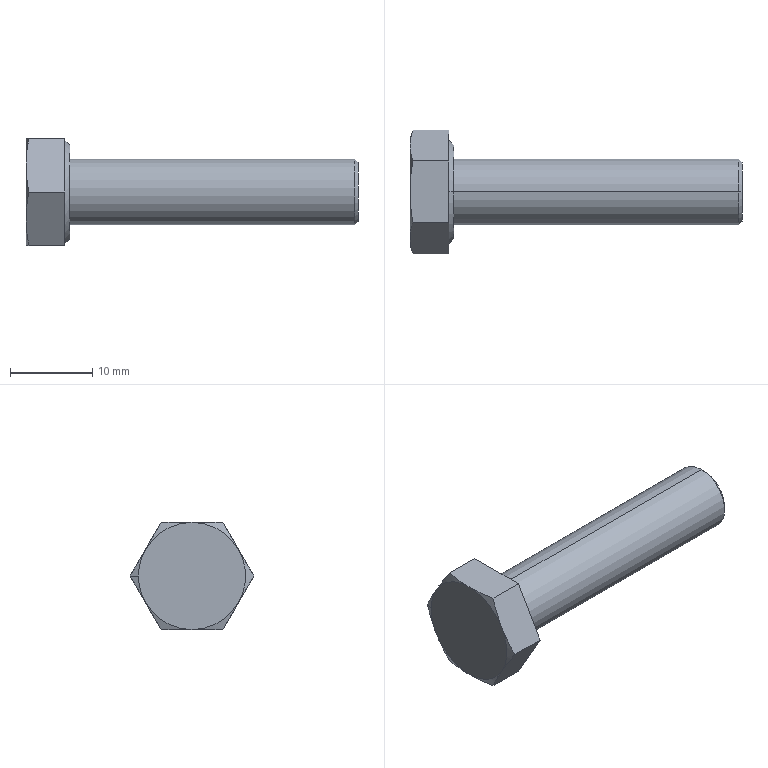Part | STEP file | hex head bolts-full thread grade c gb_GB_FASTENER_BOLT_HHBFTC M8X35-S | 1 solid | 23 faces | box 40.3 x 15.011 x 13 mm | volume 2512 mm3 | cone 11 | plane 10 | cylinder 2 | commonest cylinder face diameters 8 x2
STEP:
#1=CARTESIAN_POINT('',(39.9,0.,4.));
#2=VERTEX_POINT('',#1);
#3=CARTESIAN_POINT('',(39.9,0.,-4.));
#4=VERTEX_POINT('',#3);
#5=CARTESIAN_POINT('',(39.9,0.,0.));
#6=DIRECTION('',(-1.,0.,0.));
#7=DIRECTION('',(0.,0.,1.));
#8=AXIS2_PLACEMENT_3D('',#5,#6,#7);
#9=CIRCLE('',#8,4.);
#10=EDGE_CURVE('',#2,#4,#9,.T.);
#11=ORIENTED_EDGE('',*,*,#10,.T.);
#12=CARTESIAN_POINT('',(5.3,0.,-4.));
#13=VERTEX_POINT('',#12);
#14=CARTESIAN_POINT('',(40.3,0.,-4.));
#15=DIRECTION('',(-1.,0.,0.));
#16=VECTOR('',#15,1000.);
#17=LINE('',#14,#16);
#18=EDGE_CURVE('',#4,#13,#17,.T.);
#19=ORIENTED_EDGE('',*,*,#18,.T.);
#20=CARTESIAN_POINT('',(5.3,0.,4.));
#21=VERTEX_POINT('',#20);
#22=CARTESIAN_POINT('',(5.3,0.,0.));
#23=DIRECTION('',(1.,0.,0.));
#24=DIRECTION('',(0.,0.,1.));
#25=AXIS2_PLACEMENT_3D('',#22,#23,#24);
#26=CIRCLE('',#25,4.);
#27=EDGE_CURVE('',#13,#21,#26,.T.);
#28=ORIENTED_EDGE('',*,*,#27,.T.);
#29=CARTESIAN_POINT('',(40.3,0.,4.));
#30=DIRECTION('',(-1.,0.,0.));
#31=VECTOR('',#30,1000.);
#32=LINE('',#29,#31);
#33=EDGE_CURVE('',#2,#21,#32,.T.);
#34=ORIENTED_EDGE('',*,*,#33,.F.);
#35=EDGE_LOOP('',(#11,#19,#28,#34));
#36=FACE_OUTER_BOUND('',#35,.T.);
#37=CARTESIAN_POINT('',(40.3,0.,0.));
#38=DIRECTION('',(-1.,0.,0.));
#39=DIRECTION('',(0.,0.,1.));
#40=AXIS2_PLACEMENT_3D('',#37,#38,#39);
#41=CYLINDRICAL_SURFACE('',#40,4.);
#42=ADVANCED_FACE('',(#36),#41,.T.);
#43=CARTESIAN_POINT('',(40.3,0.,3.6));
#44=VERTEX_POINT('',#43);
#45=CARTESIAN_POINT('',(40.3,0.,-3.6));
#46=VERTEX_POINT('',#45);
#47=CARTESIAN_POINT('',(40.3,0.,0.));
#48=DIRECTION('',(-1.,0.,0.));
#49=DIRECTION('',(0.,0.,1.));
#50=AXIS2_PLACEMENT_3D('',#47,#48,#49);
#51=CIRCLE('',#50,3.6);
#52=EDGE_CURVE('',#44,#46,#51,.T.);
#53=ORIENTED_EDGE('',*,*,#52,.T.);
#54=CARTESIAN_POINT('',(39.9,0.,-4.));
#55=DIRECTION('',(-0.7071,0.,-0.7071));
#56=VECTOR('',#55,1000.);
#57=LINE('',#54,#56);
#58=EDGE_CURVE('',#46,#4,#57,.T.);
#59=ORIENTED_EDGE('',*,*,#58,.T.);
#60=ORIENTED_EDGE('',*,*,#10,.F.);
#61=CARTESIAN_POINT('',(39.9,0.,4.));
#62=DIRECTION('',(-0.7071,0.,0.7071));
#63=VECTOR('',#62,1000.);
#64=LINE('',#61,#63);
#65=EDGE_CURVE('',#44,#2,#64,.T.);
#66=ORIENTED_EDGE('',*,*,#65,.F.);
#67=EDGE_LOOP('',(#53,#59,#60,#66));
#68=FACE_OUTER_BOUND('',#67,.T.);
#69=CARTESIAN_POINT('',(39.9,0.,0.));
#70=DIRECTION('',(-1.,0.,0.));
#71=DIRECTION('',(0.,0.,1.));
#72=AXIS2_PLACEMENT_3D('',#69,#70,#71);
#73=CONICAL_SURFACE('',#72,4.,0.7854);
#74=ADVANCED_FACE('',(#68),#73,.T.);
#75=CARTESIAN_POINT('',(5.3,0.,-5.735));
#76=VERTEX_POINT('',#75);
#77=CARTESIAN_POINT('',(5.3,0.,5.735));
#78=VERTEX_POINT('',#77);
#79=CARTESIAN_POINT('',(5.3,0.,0.));
#80=DIRECTION('',(1.,0.,0.));
#81=DIRECTION('',(0.,0.,1.));
#82=AXIS2_PLACEMENT_3D('',#79,#80,#81);
#83=CIRCLE('',#82,5.735);
#84=EDGE_CURVE('',#76,#78,#83,.T.);
#85=ORIENTED_EDGE('',*,*,#84,.F.);
#86=CARTESIAN_POINT('',(4.7,0.,-6.335));
#87=VERTEX_POINT('',#86);
#88=CARTESIAN_POINT('',(4.7,0.,-6.335));
#89=DIRECTION('',(-0.7071,0.,-0.7071));
#90=VECTOR('',#89,1000.);
#91=LINE('',#88,#90);
#92=EDGE_CURVE('',#76,#87,#91,.T.);
#93=ORIENTED_EDGE('',*,*,#92,.T.);
#94=CARTESIAN_POINT('',(4.7,0.,6.335));
#95=VERTEX_POINT('',#94);
#96=CARTESIAN_POINT('',(4.7,0.,0.));
#97=DIRECTION('',(1.,0.,0.));
#98=DIRECTION('',(0.,0.,1.));
#99=AXIS2_PLACEMENT_3D('',#96,#97,#98);
#100=CIRCLE('',#99,6.335);
#101=EDGE_CURVE('',#87,#95,#100,.T.);
#102=ORIENTED_EDGE('',*,*,#101,.T.);
#103=CARTESIAN_POINT('',(4.7,0.,6.335));
#104=DIRECTION('',(-0.7071,0.,0.7071));
#105=VECTOR('',#104,1000.);
#106=LINE('',#103,#105);
#107=EDGE_CURVE('',#78,#95,#106,.T.);
#108=ORIENTED_EDGE('',*,*,#107,.F.);
#109=EDGE_LOOP('',(#85,#93,#102,#108));
#110=FACE_OUTER_BOUND('',#109,.T.);
#111=CARTESIAN_POINT('',(4.7,0.,0.));
#112=DIRECTION('',(-1.,0.,0.));
#113=DIRECTION('',(0.,0.,1.));
#114=AXIS2_PLACEMENT_3D('',#111,#112,#113);
#115=CONICAL_SURFACE('',#114,6.335,0.7854);
#116=ADVANCED_FACE('',(#110),#115,.T.);
#117=CARTESIAN_POINT('',(0.,5.629,-3.25));
#118=VERTEX_POINT('',#117);
#119=CARTESIAN_POINT('',(0.,6.5,0.));
#120=VERTEX_POINT('',#119);
#121=CARTESIAN_POINT('',(0.,0.,0.));
#122=DIRECTION('',(1.,0.,0.));
#123=DIRECTION('',(0.,1.,0.));
#124=AXIS2_PLACEMENT_3D('',#121,#122,#123);
#125=CIRCLE('',#124,6.5);
#126=EDGE_CURVE('',#118,#120,#125,.T.);
#127=ORIENTED_EDGE('',*,*,#126,.T.);
#128=CARTESIAN_POINT('',(0.366,7.506,0.));
#129=VERTEX_POINT('',#128);
#130=CARTESIAN_POINT('',(0.3682,7.512,0.));
#131=DIRECTION('',(0.342,0.9397,0.));
#132=VECTOR('',#131,1000.);
#133=LINE('',#130,#132);
#134=EDGE_CURVE('',#120,#129,#133,.T.);
#135=ORIENTED_EDGE('',*,*,#134,.T.);
#136=CARTESIAN_POINT('',(0.366,7.506,0.));
#137=CARTESIAN_POINT('',(0.1402,6.885,-1.075));
#138=CARTESIAN_POINT('',(0.,6.261,-2.156));
#139=CARTESIAN_POINT('',(0.,5.629,-3.25));
#140=B_SPLINE_CURVE_WITH_KNOTS('',3,(#136,#137,#138,#139),.UNSPECIFIED.,.F.,.F.,(4,4),(0.,0.003771),.UNSPECIFIED.);
#141=EDGE_CURVE('',#129,#118,#140,.T.);
#142=ORIENTED_EDGE('',*,*,#141,.T.);
#143=EDGE_LOOP('',(#127,#135,#142));
#144=FACE_OUTER_BOUND('',#143,.T.);
#145=CARTESIAN_POINT('',(0.3682,0.,0.));
#146=DIRECTION('',(1.,0.,0.));
#147=DIRECTION('',(0.,1.,0.));
#148=AXIS2_PLACEMENT_3D('',#145,#146,#147);
#149=CONICAL_SURFACE('',#148,7.512,1.222);
#150=ADVANCED_FACE('',(#144),#149,.T.);
#151=ORIENTED_EDGE('',*,*,#18,.F.);
#152=CARTESIAN_POINT('',(39.9,0.,0.));
#153=DIRECTION('',(-1.,0.,0.));
#154=DIRECTION('',(0.,0.,1.));
#155=AXIS2_PLACEMENT_3D('',#152,#153,#154);
#156=CIRCLE('',#155,4.);
#157=EDGE_CURVE('',#4,#2,#156,.T.);
#158=ORIENTED_EDGE('',*,*,#157,.T.);
#159=ORIENTED_EDGE('',*,*,#33,.T.);
#160=CARTESIAN_POINT('',(5.3,0.,0.));
#161=DIRECTION('',(1.,0.,0.));
#162=DIRECTION('',(0.,0.,1.));
#163=AXIS2_PLACEMENT_3D('',#160,#161,#162);
#164=CIRCLE('',#163,4.);
#165=EDGE_CURVE('',#21,#13,#164,.T.);
#166=ORIENTED_EDGE('',*,*,#165,.T.);
#167=EDGE_LOOP('',(#151,#158,#159,#166));
#168=FACE_OUTER_BOUND('',#167,.T.);
#169=CARTESIAN_POINT('',(40.3,0.,0.));
#170=DIRECTION('',(-1.,0.,0.));
#171=DIRECTION('',(0.,0.,1.));
#172=AXIS2_PLACEMENT_3D('',#169,#170,#171);
#173=CYLINDRICAL_SURFACE('',#172,4.);
#174=ADVANCED_FACE('',(#168),#173,.T.);
#175=ORIENTED_EDGE('',*,*,#165,.F.);
#176=ORIENTED_EDGE('',*,*,#27,.F.);
#177=EDGE_LOOP('',(#175,#176));
#178=FACE_BOUND('',#177,.T.);
#179=CARTESIAN_POINT('',(5.3,0.,0.));
#180=DIRECTION('',(1.,0.,0.));
#181=DIRECTION('',(0.,0.,1.));
#182=AXIS2_PLACEMENT_3D('',#179,#180,#181);
#183=CIRCLE('',#182,5.735);
#184=EDGE_CURVE('',#78,#76,#183,.T.);
#185=ORIENTED_EDGE('',*,*,#184,.T.);
#186=ORIENTED_EDGE('',*,*,#84,.T.);
#187=EDGE_LOOP('',(#185,#186));
#188=FACE_OUTER_BOUND('',#187,.T.);
#189=CARTESIAN_POINT('',(5.3,-7.506,0.));
#190=DIRECTION('',(1.,0.,0.));
#191=DIRECTION('',(0.,0.,-1.));
#192=AXIS2_PLACEMENT_3D('',#189,#190,#191);
#193=PLANE('',#192);
#194=ADVANCED_FACE('',(#178,#188),#193,.T.);
#195=ORIENTED_EDGE('',*,*,#58,.F.);
#196=CARTESIAN_POINT('',(40.3,0.,0.));
#197=DIRECTION('',(-1.,0.,0.));
#198=DIRECTION('',(0.,0.,1.));
#199=AXIS2_PLACEMENT_3D('',#196,#197,#198);
#200=CIRCLE('',#199,3.6);
#201=EDGE_CURVE('',#46,#44,#200,.T.);
#202=ORIENTED_EDGE('',*,*,#201,.T.);
#203=ORIENTED_EDGE('',*,*,#65,.T.);
#204=ORIENTED_EDGE('',*,*,#157,.F.);
#205=EDGE_LOOP('',(#195,#202,#203,#204));
#206=FACE_OUTER_BOUND('',#205,.T.);
#207=CARTESIAN_POINT('',(39.9,0.,0.));
#208=DIRECTION('',(-1.,0.,0.));
#209=DIRECTION('',(0.,0.,1.));
#210=AXIS2_PLACEMENT_3D('',#207,#208,#209);
#211=CONICAL_SURFACE('',#210,4.,0.7854);
#212=ADVANCED_FACE('',(#206),#211,.T.);
#213=ORIENTED_EDGE('',*,*,#92,.F.);
#214=ORIENTED_EDGE('',*,*,#184,.F.);
#215=ORIENTED_EDGE('',*,*,#107,.T.);
#216=CARTESIAN_POINT('',(4.7,0.,0.));
#217=DIRECTION('',(1.,0.,0.));
#218=DIRECTION('',(0.,0.,1.));
#219=AXIS2_PLACEMENT_3D('',#216,#217,#218);
#220=CIRCLE('',#219,6.335);
#221=EDGE_CURVE('',#95,#87,#220,.T.);
#222=ORIENTED_EDGE('',*,*,#221,.T.);
#223=EDGE_LOOP('',(#213,#214,#215,#222));
#224=FACE_OUTER_BOUND('',#223,.T.);
#225=CARTESIAN_POINT('',(4.7,0.,0.));
#226=DIRECTION('',(-1.,0.,0.));
#227=DIRECTION('',(0.,0.,1.));
#228=AXIS2_PLACEMENT_3D('',#225,#226,#227);
#229=CONICAL_SURFACE('',#228,6.335,0.7854);
#230=ADVANCED_FACE('',(#224),#229,.T.);
#231=ORIENTED_EDGE('',*,*,#52,.F.);
#232=ORIENTED_EDGE('',*,*,#201,.F.);
#233=EDGE_LOOP('',(#231,#232));
#234=FACE_OUTER_BOUND('',#233,.T.);
#235=CARTESIAN_POINT('',(40.3,0.,0.));
#236=DIRECTION('',(1.,0.,0.));
#237=DIRECTION('',(0.,0.,-1.));
#238=AXIS2_PLACEMENT_3D('',#235,#236,#237);
#239=PLANE('',#238);
#240=ADVANCED_FACE('',(#234),#239,.T.);
#241=CARTESIAN_POINT('',(4.7,7.506,0.));
#242=VERTEX_POINT('',#241);
#243=CARTESIAN_POINT('',(4.7,3.753,6.5));
#244=VERTEX_POINT('',#243);
#245=CARTESIAN_POINT('',(4.7,7.506,0.));
#246=DIRECTION('',(0.,-0.5,0.866));
#247=VECTOR('',#246,1000.);
#248=LINE('',#245,#247);
#249=EDGE_CURVE('',#242,#244,#248,.T.);
#250=ORIENTED_EDGE('',*,*,#249,.T.);
#251=CARTESIAN_POINT('',(4.7,-3.753,6.5));
#252=VERTEX_POINT('',#251);
#253=CARTESIAN_POINT('',(4.7,6.335,6.5));
#254=DIRECTION('',(0.,-1.,0.));
#255=VECTOR('',#254,1000.);
#256=LINE('',#253,#255);
#257=EDGE_CURVE('',#244,#252,#256,.T.);
#258=ORIENTED_EDGE('',*,*,#257,.T.);
#259=CARTESIAN_POINT('',(4.7,-7.506,0.));
#260=VERTEX_POINT('',#259);
#261=CARTESIAN_POINT('',(4.7,-3.753,6.5));
#262=DIRECTION('',(0.,-0.5,-0.866));
#263=VECTOR('',#262,1000.);
#264=LINE('',#261,#263);
#265=EDGE_CURVE('',#252,#260,#264,.T.);
#266=ORIENTED_EDGE('',*,*,#265,.T.);
#267=CARTESIAN_POINT('',(4.7,-3.753,-6.5));
#268=VERTEX_POINT('',#267);
#269=CARTESIAN_POINT('',(4.7,-7.506,0.));
#270=DIRECTION('',(0.,0.5,-0.866));
#271=VECTOR('',#270,1000.);
#272=LINE('',#269,#271);
#273=EDGE_CURVE('',#260,#268,#272,.T.);
#274=ORIENTED_EDGE('',*,*,#273,.T.);
#275=CARTESIAN_POINT('',(4.7,3.753,-6.5));
#276=VERTEX_POINT('',#275);
#277=CARTESIAN_POINT('',(4.7,6.335,-6.5));
#278=DIRECTION('',(0.,1.,0.));
#279=VECTOR('',#278,1000.);
#280=LINE('',#277,#279);
#281=EDGE_CURVE('',#268,#276,#280,.T.);
#282=ORIENTED_EDGE('',*,*,#281,.T.);
#283=CARTESIAN_POINT('',(4.7,3.753,-6.5));
#284=DIRECTION('',(0.,0.5,0.866));
#285=VECTOR('',#284,1000.);
#286=LINE('',#283,#285);
#287=EDGE_CURVE('',#276,#242,#286,.T.);
#288=ORIENTED_EDGE('',*,*,#287,.T.);
#289=EDGE_LOOP('',(#250,#258,#266,#274,#282,#288));
#290=FACE_OUTER_BOUND('',#289,.T.);
#291=ORIENTED_EDGE('',*,*,#221,.F.);
#292=ORIENTED_EDGE('',*,*,#101,.F.);
#293=EDGE_LOOP('',(#291,#292));
#294=FACE_BOUND('',#293,.T.);
#295=CARTESIAN_POINT('',(4.7,6.335,0.));
#296=DIRECTION('',(1.,0.,0.));
#297=DIRECTION('',(0.,0.,-1.));
#298=AXIS2_PLACEMENT_3D('',#295,#296,#297);
#299=PLANE('',#298);
#300=ADVANCED_FACE('',(#290,#294),#299,.T.);
#301=CARTESIAN_POINT('',(0.366,-3.753,6.5));
#302=VERTEX_POINT('',#301);
#303=CARTESIAN_POINT('',(5.3,-3.753,6.5));
#304=DIRECTION('',(-1.,0.,0.));
#305=VECTOR('',#304,1000.);
#306=LINE('',#303,#305);
#307=EDGE_CURVE('',#252,#302,#306,.T.);
#308=ORIENTED_EDGE('',*,*,#307,.F.);
#309=ORIENTED_EDGE('',*,*,#257,.F.);
#310=CARTESIAN_POINT('',(0.366,3.753,6.5));
#311=VERTEX_POINT('',#310);
#312=CARTESIAN_POINT('',(5.3,3.753,6.5));
#313=DIRECTION('',(1.,0.,0.));
#314=VECTOR('',#313,1000.);
#315=LINE('',#312,#314);
#316=EDGE_CURVE('',#311,#244,#315,.T.);
#317=ORIENTED_EDGE('',*,*,#316,.F.);
#318=CARTESIAN_POINT('',(0.,0.,6.5));
#319=VERTEX_POINT('',#318);
#320=CARTESIAN_POINT('',(0.,0.,6.5));
#321=CARTESIAN_POINT('',(0.,1.263,6.5));
#322=CARTESIAN_POINT('',(0.1402,2.512,6.5));
#323=CARTESIAN_POINT('',(0.366,3.753,6.5));
#324=B_SPLINE_CURVE_WITH_KNOTS('',3,(#320,#321,#322,#323),.UNSPECIFIED.,.F.,.F.,(4,4),(0.,0.003771),.UNSPECIFIED.);
#325=EDGE_CURVE('',#319,#311,#324,.T.);
#326=ORIENTED_EDGE('',*,*,#325,.F.);
#327=CARTESIAN_POINT('',(0.366,-3.753,6.5));
#328=CARTESIAN_POINT('',(0.1402,-2.512,6.5));
#329=CARTESIAN_POINT('',(0.,-1.263,6.5));
#330=CARTESIAN_POINT('',(0.,0.,6.5));
#331=B_SPLINE_CURVE_WITH_KNOTS('',3,(#327,#328,#329,#330),.UNSPECIFIED.,.F.,.F.,(4,4),(0.,0.003771),.UNSPECIFIED.);
#332=EDGE_CURVE('',#302,#319,#331,.T.);
#333=ORIENTED_EDGE('',*,*,#332,.F.);
#334=EDGE_LOOP('',(#308,#309,#317,#326,#333));
#335=FACE_OUTER_BOUND('',#334,.T.);
#336=CARTESIAN_POINT('',(5.3,3.753,6.5));
#337=DIRECTION('',(0.,0.,-1.));
#338=DIRECTION('',(-1.,0.,0.));
#339=AXIS2_PLACEMENT_3D('',#336,#337,#338);
#340=PLANE('',#339);
#341=ADVANCED_FACE('',(#335),#340,.F.);
#342=ORIENTED_EDGE('',*,*,#316,.T.);
#343=ORIENTED_EDGE('',*,*,#249,.F.);
#344=CARTESIAN_POINT('',(5.3,7.506,0.));
#345=DIRECTION('',(1.,0.,0.));
#346=VECTOR('',#345,1000.);
#347=LINE('',#344,#346);
#348=EDGE_CURVE('',#129,#242,#347,.T.);
#349=ORIENTED_EDGE('',*,*,#348,.F.);
#350=CARTESIAN_POINT('',(0.,5.629,3.25));
#351=VERTEX_POINT('',#350);
#352=CARTESIAN_POINT('',(0.,5.629,3.25));
#353=CARTESIAN_POINT('',(0.,6.261,2.156));
#354=CARTESIAN_POINT('',(0.1402,6.885,1.075));
#355=CARTESIAN_POINT('',(0.366,7.506,0.));
#356=B_SPLINE_CURVE_WITH_KNOTS('',3,(#352,#353,#354,#355),.UNSPECIFIED.,.F.,.F.,(4,4),(0.,0.003771),.UNSPECIFIED.);
#357=EDGE_CURVE('',#351,#129,#356,.T.);
#358=ORIENTED_EDGE('',*,*,#357,.F.);
#359=CARTESIAN_POINT('',(0.366,3.753,6.5));
#360=CARTESIAN_POINT('',(0.1402,4.373,5.425));
#361=CARTESIAN_POINT('',(0.,4.998,4.344));
#362=CARTESIAN_POINT('',(0.,5.629,3.25));
#363=B_SPLINE_CURVE_WITH_KNOTS('',3,(#359,#360,#361,#362),.UNSPECIFIED.,.F.,.F.,(4,4),(0.,0.003771),.UNSPECIFIED.);
#364=EDGE_CURVE('',#311,#351,#363,.T.);
#365=ORIENTED_EDGE('',*,*,#364,.F.);
#366=EDGE_LOOP('',(#342,#343,#349,#358,#365));
#367=FACE_OUTER_BOUND('',#366,.T.);
#368=CARTESIAN_POINT('',(5.3,7.506,0.));
#369=DIRECTION('',(0.,-0.866,-0.5));
#370=DIRECTION('',(0.,0.5,-0.866));
#371=AXIS2_PLACEMENT_3D('',#368,#369,#370);
#372=PLANE('',#371);
#373=ADVANCED_FACE('',(#367),#372,.F.);
#374=ORIENTED_EDGE('',*,*,#348,.T.);
#375=ORIENTED_EDGE('',*,*,#287,.F.);
#376=CARTESIAN_POINT('',(0.366,3.753,-6.5));
#377=VERTEX_POINT('',#376);
#378=CARTESIAN_POINT('',(5.3,3.753,-6.5));
#379=DIRECTION('',(1.,0.,0.));
#380=VECTOR('',#379,1000.);
#381=LINE('',#378,#380);
#382=EDGE_CURVE('',#377,#276,#381,.T.);
#383=ORIENTED_EDGE('',*,*,#382,.F.);
#384=CARTESIAN_POINT('',(0.,5.629,-3.25));
#385=CARTESIAN_POINT('',(0.,4.998,-4.344));
#386=CARTESIAN_POINT('',(0.1402,4.373,-5.425));
#387=CARTESIAN_POINT('',(0.366,3.753,-6.5));
#388=B_SPLINE_CURVE_WITH_KNOTS('',3,(#384,#385,#386,#387),.UNSPECIFIED.,.F.,.F.,(4,4),(0.,0.003771),.UNSPECIFIED.);
#389=EDGE_CURVE('',#118,#377,#388,.T.);
#390=ORIENTED_EDGE('',*,*,#389,.F.);
#391=ORIENTED_EDGE('',*,*,#141,.F.);
#392=EDGE_LOOP('',(#374,#375,#383,#390,#391));
#393=FACE_OUTER_BOUND('',#392,.T.);
#394=CARTESIAN_POINT('',(5.3,3.753,-6.5));
#395=DIRECTION('',(0.,-0.866,0.5));
#396=DIRECTION('',(0.,-0.5,-0.866));
#397=AXIS2_PLACEMENT_3D('',#394,#395,#396);
#398=PLANE('',#397);
#399=ADVANCED_FACE('',(#393),#398,.F.);
#400=ORIENTED_EDGE('',*,*,#382,.T.);
#401=ORIENTED_EDGE('',*,*,#281,.F.);
#402=CARTESIAN_POINT('',(0.366,-3.753,-6.5));
#403=VERTEX_POINT('',#402);
#404=CARTESIAN_POINT('',(5.3,-3.753,-6.5));
#405=DIRECTION('',(1.,0.,0.));
#406=VECTOR('',#405,1000.);
#407=LINE('',#404,#406);
#408=EDGE_CURVE('',#403,#268,#407,.T.);
#409=ORIENTED_EDGE('',*,*,#408,.F.);
#410=CARTESIAN_POINT('',(0.,0.,-6.5));
#411=VERTEX_POINT('',#410);
#412=CARTESIAN_POINT('',(0.,0.,-6.5));
#413=CARTESIAN_POINT('',(0.,-1.263,-6.5));
#414=CARTESIAN_POINT('',(0.1402,-2.512,-6.5));
#415=CARTESIAN_POINT('',(0.366,-3.753,-6.5));
#416=B_SPLINE_CURVE_WITH_KNOTS('',3,(#412,#413,#414,#415),.UNSPECIFIED.,.F.,.F.,(4,4),(0.,0.003771),.UNSPECIFIED.);
#417=EDGE_CURVE('',#411,#403,#416,.T.);
#418=ORIENTED_EDGE('',*,*,#417,.F.);
#419=CARTESIAN_POINT('',(0.366,3.753,-6.5));
#420=CARTESIAN_POINT('',(0.1402,2.512,-6.5));
#421=CARTESIAN_POINT('',(0.,1.263,-6.5));
#422=CARTESIAN_POINT('',(0.,0.,-6.5));
#423=B_SPLINE_CURVE_WITH_KNOTS('',3,(#419,#420,#421,#422),.UNSPECIFIED.,.F.,.F.,(4,4),(0.,0.003771),.UNSPECIFIED.);
#424=EDGE_CURVE('',#377,#411,#423,.T.);
#425=ORIENTED_EDGE('',*,*,#424,.F.);
#426=EDGE_LOOP('',(#400,#401,#409,#418,#425));
#427=FACE_OUTER_BOUND('',#426,.T.);
#428=CARTESIAN_POINT('',(5.3,-3.753,-6.5));
#429=DIRECTION('',(0.,0.,1.));
#430=DIRECTION('',(0.,-1.,0.));
#431=AXIS2_PLACEMENT_3D('',#428,#429,#430);
#432=PLANE('',#431);
#433=ADVANCED_FACE('',(#427),#432,.F.);
#434=ORIENTED_EDGE('',*,*,#408,.T.);
#435=ORIENTED_EDGE('',*,*,#273,.F.);
#436=CARTESIAN_POINT('',(0.366,-7.506,0.));
#437=VERTEX_POINT('',#436);
#438=CARTESIAN_POINT('',(5.3,-7.506,0.));
#439=DIRECTION('',(1.,0.,0.));
#440=VECTOR('',#439,1000.);
#441=LINE('',#438,#440);
#442=EDGE_CURVE('',#437,#260,#441,.T.);
#443=ORIENTED_EDGE('',*,*,#442,.F.);
#444=CARTESIAN_POINT('',(0.,-5.629,-3.25));
#445=VERTEX_POINT('',#444);
#446=CARTESIAN_POINT('',(0.,-5.629,-3.25));
#447=CARTESIAN_POINT('',(0.,-6.261,-2.156));
#448=CARTESIAN_POINT('',(0.1402,-6.885,-1.075));
#449=CARTESIAN_POINT('',(0.366,-7.506,0.));
#450=B_SPLINE_CURVE_WITH_KNOTS('',3,(#446,#447,#448,#449),.UNSPECIFIED.,.F.,.F.,(4,4),(0.,0.003771),.UNSPECIFIED.);
#451=EDGE_CURVE('',#445,#437,#450,.T.);
#452=ORIENTED_EDGE('',*,*,#451,.F.);
#453=CARTESIAN_POINT('',(0.366,-3.753,-6.5));
#454=CARTESIAN_POINT('',(0.1402,-4.373,-5.425));
#455=CARTESIAN_POINT('',(0.,-4.998,-4.344));
#456=CARTESIAN_POINT('',(0.,-5.629,-3.25));
#457=B_SPLINE_CURVE_WITH_KNOTS('',3,(#453,#454,#455,#456),.UNSPECIFIED.,.F.,.F.,(4,4),(0.,0.003771),.UNSPECIFIED.);
#458=EDGE_CURVE('',#403,#445,#457,.T.);
#459=ORIENTED_EDGE('',*,*,#458,.F.);
#460=EDGE_LOOP('',(#434,#435,#443,#452,#459));
#461=FACE_OUTER_BOUND('',#460,.T.);
#462=CARTESIAN_POINT('',(5.3,-7.506,0.));
#463=DIRECTION('',(0.,0.866,0.5));
#464=DIRECTION('',(0.,-0.5,0.866));
#465=AXIS2_PLACEMENT_3D('',#462,#463,#464);
#466=PLANE('',#465);
#467=ADVANCED_FACE('',(#461),#466,.F.);
#468=ORIENTED_EDGE('',*,*,#442,.T.);
#469=ORIENTED_EDGE('',*,*,#265,.F.);
#470=ORIENTED_EDGE('',*,*,#307,.T.);
#471=CARTESIAN_POINT('',(0.,-5.629,3.25));
#472=VERTEX_POINT('',#471);
#473=CARTESIAN_POINT('',(0.,-5.629,3.25));
#474=CARTESIAN_POINT('',(0.,-4.998,4.344));
#475=CARTESIAN_POINT('',(0.1402,-4.373,5.425));
#476=CARTESIAN_POINT('',(0.366,-3.753,6.5));
#477=B_SPLINE_CURVE_WITH_KNOTS('',3,(#473,#474,#475,#476),.UNSPECIFIED.,.F.,.F.,(4,4),(0.,0.003771),.UNSPECIFIED.);
#478=EDGE_CURVE('',#472,#302,#477,.T.);
#479=ORIENTED_EDGE('',*,*,#478,.F.);
#480=CARTESIAN_POINT('',(0.366,-7.506,0.));
#481=CARTESIAN_POINT('',(0.1402,-6.885,1.075));
#482=CARTESIAN_POINT('',(0.,-6.261,2.156));
#483=CARTESIAN_POINT('',(0.,-5.629,3.25));
#484=B_SPLINE_CURVE_WITH_KNOTS('',3,(#480,#481,#482,#483),.UNSPECIFIED.,.F.,.F.,(4,4),(0.,0.003771),.UNSPECIFIED.);
#485=EDGE_CURVE('',#437,#472,#484,.T.);
#486=ORIENTED_EDGE('',*,*,#485,.F.);
#487=EDGE_LOOP('',(#468,#469,#470,#479,#486));
#488=FACE_OUTER_BOUND('',#487,.T.);
#489=CARTESIAN_POINT('',(5.3,-3.753,6.5));
#490=DIRECTION('',(0.,0.866,-0.5));
#491=DIRECTION('',(0.,0.5,0.866));
#492=AXIS2_PLACEMENT_3D('',#489,#490,#491);
#493=PLANE('',#492);
#494=ADVANCED_FACE('',(#488),#493,.F.);
#495=ORIENTED_EDGE('',*,*,#332,.T.);
#496=CARTESIAN_POINT('',(0.,0.,0.));
#497=DIRECTION('',(1.,0.,0.));
#498=DIRECTION('',(0.,1.,0.));
#499=AXIS2_PLACEMENT_3D('',#496,#497,#498);
#500=CIRCLE('',#499,6.5);
#501=EDGE_CURVE('',#319,#472,#500,.T.);
#502=ORIENTED_EDGE('',*,*,#501,.T.);
#503=ORIENTED_EDGE('',*,*,#478,.T.);
#504=EDGE_LOOP('',(#495,#502,#503));
#505=FACE_OUTER_BOUND('',#504,.T.);
#506=CARTESIAN_POINT('',(0.3682,0.,0.));
#507=DIRECTION('',(1.,0.,0.));
#508=DIRECTION('',(0.,1.,0.));
#509=AXIS2_PLACEMENT_3D('',#506,#507,#508);
#510=CONICAL_SURFACE('',#509,7.512,1.222);
#511=ADVANCED_FACE('',(#505),#510,.T.);
#512=CARTESIAN_POINT('',(0.,0.,0.));
#513=DIRECTION('',(1.,0.,0.));
#514=DIRECTION('',(0.,1.,0.));
#515=AXIS2_PLACEMENT_3D('',#512,#513,#514);
#516=CIRCLE('',#515,6.5);
#517=EDGE_CURVE('',#351,#319,#516,.T.);
#518=ORIENTED_EDGE('',*,*,#517,.T.);
#519=ORIENTED_EDGE('',*,*,#325,.T.);
#520=ORIENTED_EDGE('',*,*,#364,.T.);
#521=EDGE_LOOP('',(#518,#519,#520));
#522=FACE_OUTER_BOUND('',#521,.T.);
#523=CARTESIAN_POINT('',(0.3682,0.,0.));
#524=DIRECTION('',(1.,0.,0.));
#525=DIRECTION('',(0.,1.,0.));
#526=AXIS2_PLACEMENT_3D('',#523,#524,#525);
#527=CONICAL_SURFACE('',#526,7.512,1.222);
#528=ADVANCED_FACE('',(#522),#527,.T.);
#529=ORIENTED_EDGE('',*,*,#134,.F.);
#530=CARTESIAN_POINT('',(0.,0.,0.));
#531=DIRECTION('',(1.,0.,0.));
#532=DIRECTION('',(0.,1.,0.));
#533=AXIS2_PLACEMENT_3D('',#530,#531,#532);
#534=CIRCLE('',#533,6.5);
#535=EDGE_CURVE('',#120,#351,#534,.T.);
#536=ORIENTED_EDGE('',*,*,#535,.T.);
#537=ORIENTED_EDGE('',*,*,#357,.T.);
#538=EDGE_LOOP('',(#529,#536,#537));
#539=FACE_OUTER_BOUND('',#538,.T.);
#540=CARTESIAN_POINT('',(0.3682,0.,0.));
#541=DIRECTION('',(1.,0.,0.));
#542=DIRECTION('',(0.,1.,0.));
#543=AXIS2_PLACEMENT_3D('',#540,#541,#542);
#544=CONICAL_SURFACE('',#543,7.512,1.222);
#545=ADVANCED_FACE('',(#539),#544,.T.);
#546=CARTESIAN_POINT('',(0.,0.,0.));
#547=DIRECTION('',(1.,0.,0.));
#548=DIRECTION('',(0.,1.,0.));
#549=AXIS2_PLACEMENT_3D('',#546,#547,#548);
#550=CIRCLE('',#549,6.5);
#551=EDGE_CURVE('',#411,#118,#550,.T.);
#552=ORIENTED_EDGE('',*,*,#551,.T.);
#553=ORIENTED_EDGE('',*,*,#389,.T.);
#554=ORIENTED_EDGE('',*,*,#424,.T.);
#555=EDGE_LOOP('',(#552,#553,#554));
#556=FACE_OUTER_BOUND('',#555,.T.);
#557=CARTESIAN_POINT('',(0.3682,0.,0.));
#558=DIRECTION('',(1.,0.,0.));
#559=DIRECTION('',(0.,1.,0.));
#560=AXIS2_PLACEMENT_3D('',#557,#558,#559);
#561=CONICAL_SURFACE('',#560,7.512,1.222);
#562=ADVANCED_FACE('',(#556),#561,.T.);
#563=ORIENTED_EDGE('',*,*,#458,.T.);
#564=CARTESIAN_POINT('',(0.,0.,0.));
#565=DIRECTION('',(1.,0.,0.));
#566=DIRECTION('',(0.,1.,0.));
#567=AXIS2_PLACEMENT_3D('',#564,#565,#566);
#568=CIRCLE('',#567,6.5);
#569=EDGE_CURVE('',#445,#411,#568,.T.);
#570=ORIENTED_EDGE('',*,*,#569,.T.);
#571=ORIENTED_EDGE('',*,*,#417,.T.);
#572=EDGE_LOOP('',(#563,#570,#571));
#573=FACE_OUTER_BOUND('',#572,.T.);
#574=CARTESIAN_POINT('',(0.3682,0.,0.));
#575=DIRECTION('',(1.,0.,0.));
#576=DIRECTION('',(0.,1.,0.));
#577=AXIS2_PLACEMENT_3D('',#574,#575,#576);
#578=CONICAL_SURFACE('',#577,7.512,1.222);
#579=ADVANCED_FACE('',(#573),#578,.T.);
#580=ORIENTED_EDGE('',*,*,#485,.T.);
#581=CARTESIAN_POINT('',(0.,0.,0.));
#582=DIRECTION('',(1.,0.,0.));
#583=DIRECTION('',(0.,1.,0.));
#584=AXIS2_PLACEMENT_3D('',#581,#582,#583);
#585=CIRCLE('',#584,6.5);
#586=EDGE_CURVE('',#472,#445,#585,.T.);
#587=ORIENTED_EDGE('',*,*,#586,.T.);
#588=ORIENTED_EDGE('',*,*,#451,.T.);
#589=EDGE_LOOP('',(#580,#587,#588));
#590=FACE_OUTER_BOUND('',#589,.T.);
#591=CARTESIAN_POINT('',(0.3682,0.,0.));
#592=DIRECTION('',(1.,0.,0.));
#593=DIRECTION('',(0.,1.,0.));
#594=AXIS2_PLACEMENT_3D('',#591,#592,#593);
#595=CONICAL_SURFACE('',#594,7.512,1.222);
#596=ADVANCED_FACE('',(#590),#595,.T.);
#597=ORIENTED_EDGE('',*,*,#569,.F.);
#598=ORIENTED_EDGE('',*,*,#586,.F.);
#599=ORIENTED_EDGE('',*,*,#501,.F.);
#600=ORIENTED_EDGE('',*,*,#517,.F.);
#601=ORIENTED_EDGE('',*,*,#535,.F.);
#602=ORIENTED_EDGE('',*,*,#126,.F.);
#603=ORIENTED_EDGE('',*,*,#551,.F.);
#604=EDGE_LOOP('',(#597,#598,#599,#600,#601,#602,#603));
#605=FACE_OUTER_BOUND('',#604,.T.);
#606=CARTESIAN_POINT('',(0.,-7.506,0.));
#607=DIRECTION('',(1.,0.,0.));
#608=DIRECTION('',(0.,0.,-1.));
#609=AXIS2_PLACEMENT_3D('',#606,#607,#608);
#610=PLANE('',#609);
#611=ADVANCED_FACE('',(#605),#610,.F.);
#612=CLOSED_SHELL('',(#42,#74,#116,#150,#174,#194,#212,#230,#240,#300,#341,#373,#399,#433,#467,#494,#511,#528,#545,#562,#579,#596,#611));
#613=MANIFOLD_SOLID_BREP('',#612);
#614=CARTESIAN_POINT('',(0.,0.,0.));
#615=DIRECTION('',(0.,0.,1.));
#616=DIRECTION('',(1.,0.,0.));
#617=AXIS2_PLACEMENT_3D('',#614,#615,#616);
#618=(LENGTH_UNIT()NAMED_UNIT(*)SI_UNIT(.MILLI.,.METRE.));
#619=UNCERTAINTY_MEASURE_WITH_UNIT(LENGTH_MEASURE(0.00001),#618,'','');
#620=(NAMED_UNIT(*)PLANE_ANGLE_UNIT()SI_UNIT($,.RADIAN.));
#621=(NAMED_UNIT(*)SI_UNIT($,.STERADIAN.)SOLID_ANGLE_UNIT());
#622=(GEOMETRIC_REPRESENTATION_CONTEXT(3)GLOBAL_UNCERTAINTY_ASSIGNED_CONTEXT((#619))GLOBAL_UNIT_ASSIGNED_CONTEXT((#618,#620,#621))REPRESENTATION_CONTEXT('',''));
#623=ADVANCED_BREP_SHAPE_REPRESENTATION('',(#613,#617),#622);